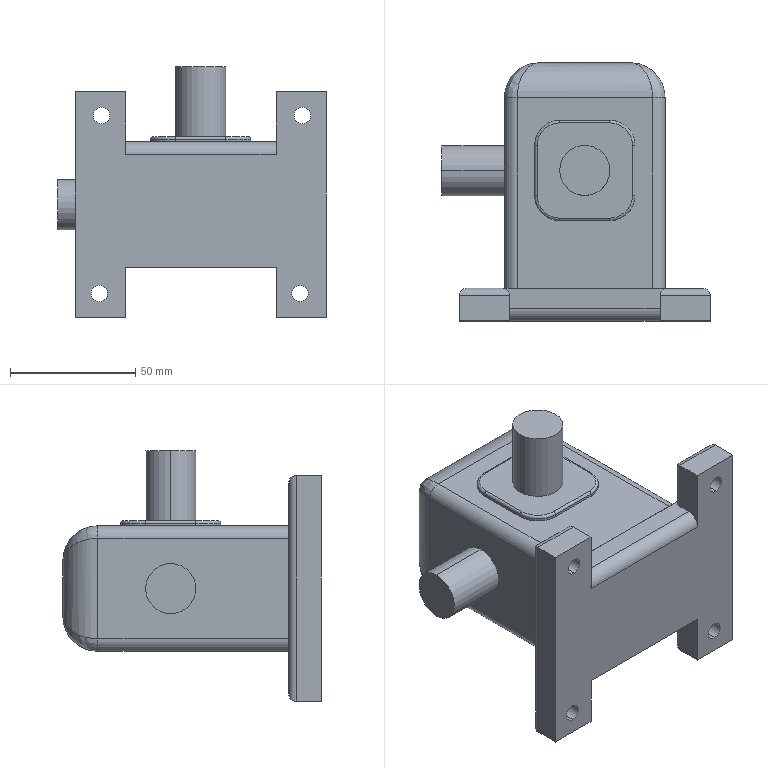Part | NX | 1 solid | 73 faces | box 107 x 103 x 99.996 mm | volume 380295 mm3 | cylinder 39 | plane 26 | torus 4 | spline 4 | commonest cylinder face diameters 6 x10 6.6 x8 20 x8 10 x5 2 x4 28 x4